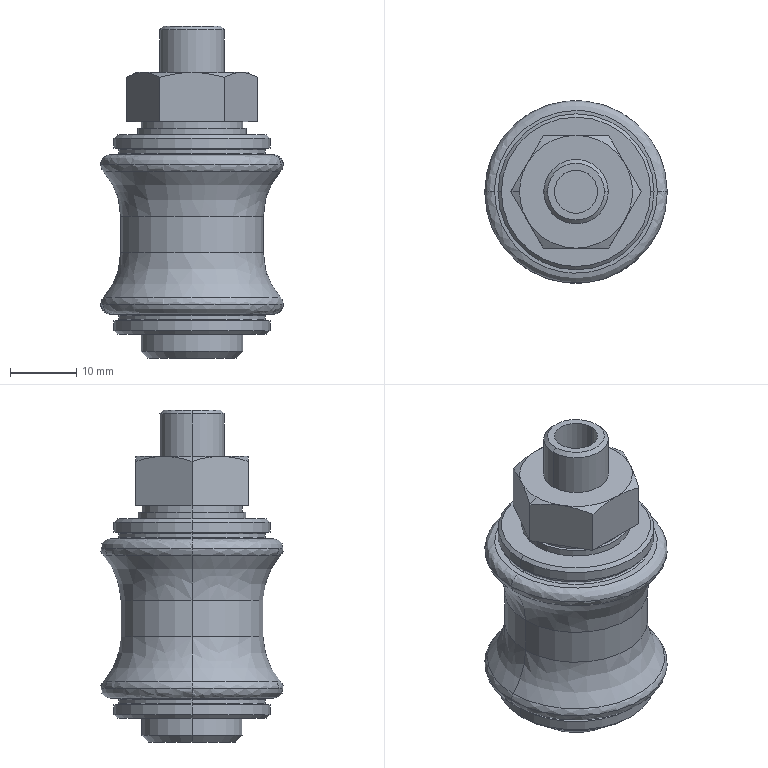Part | STEP file | Hand slide valve HSV06 | 2 solids | 85 faces | box 27.5 x 27.5 x 50 mm | volume 15432 mm3 | spline 24 | cylinder 24 | plane 20 | cone 17 | commonest cylinder face diameters 15.3 x4 16.3 x4 22.1 x4 23.5 x4 6.485 x2 8.566 x2